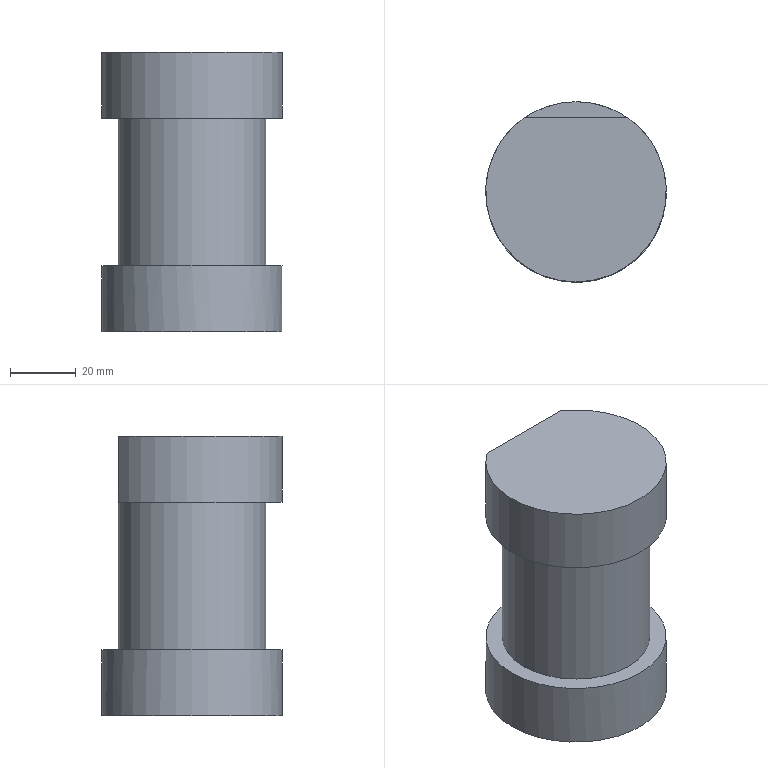Part | NX | features solid 2 | 1 solid | 11 faces | box 55 x 55 x 85 mm | volume 132305 mm3 | plane 6 | cylinder 4 | cone 1 | commonest cylinder face diameters 55 x2 24 x1 45 x1
STEP:
#1=CARTESIAN_POINT('',(690.,-642.5,100.));
#2=VERTEX_POINT('',#1);
#3=CARTESIAN_POINT('',(690.,-665.,100.));
#4=DIRECTION('',(0.,0.,1.));
#5=DIRECTION('',(1.,0.,0.));
#6=AXIS2_PLACEMENT_3D('',#3,#4,#5);
#7=CIRCLE('',#6,22.5);
#8=EDGE_CURVE('',#2,#2,#7,.T.);
#9=ORIENTED_EDGE('',*,*,#8,.F.);
#10=EDGE_LOOP('',(#9));
#11=FACE_BOUND('',#10,.T.);
#12=CARTESIAN_POINT('',(667.5,-665.,55.));
#13=VERTEX_POINT('',#12);
#14=CARTESIAN_POINT('',(690.,-665.,55.));
#15=DIRECTION('',(0.,0.,-1.));
#16=DIRECTION('',(-1.,0.,0.));
#17=AXIS2_PLACEMENT_3D('',#14,#15,#16);
#18=CIRCLE('',#17,22.5);
#19=EDGE_CURVE('',#13,#13,#18,.F.);
#20=ORIENTED_EDGE('',*,*,#19,.T.);
#21=EDGE_LOOP('',(#20));
#22=FACE_BOUND('',#21,.T.);
#23=CARTESIAN_POINT('',(690.,-665.,55.));
#24=DIRECTION('',(0.,0.,1.));
#25=DIRECTION('',(-1.,0.,0.));
#26=AXIS2_PLACEMENT_3D('',#23,#24,#25);
#27=CYLINDRICAL_SURFACE('',#26,22.5);
#28=ADVANCED_FACE('',(#11,#22),#27,.T.);
#29=ORIENTED_EDGE('',*,*,#19,.F.);
#30=EDGE_LOOP('',(#29));
#31=FACE_BOUND('',#30,.T.);
#32=CARTESIAN_POINT('',(717.5,-665.,55.));
#33=VERTEX_POINT('',#32);
#34=CARTESIAN_POINT('',(690.,-665.,55.));
#35=DIRECTION('',(0.,0.,1.));
#36=DIRECTION('',(1.,0.,0.));
#37=AXIS2_PLACEMENT_3D('',#34,#35,#36);
#38=CIRCLE('',#37,27.5);
#39=EDGE_CURVE('',#33,#33,#38,.T.);
#40=ORIENTED_EDGE('',*,*,#39,.T.);
#41=EDGE_LOOP('',(#40));
#42=FACE_BOUND('',#41,.T.);
#43=CARTESIAN_POINT('',(690.,-665.,55.));
#44=DIRECTION('',(0.,0.,1.));
#45=DIRECTION('',(-1.,0.,0.));
#46=AXIS2_PLACEMENT_3D('',#43,#44,#45);
#47=PLANE('',#46);
#48=ADVANCED_FACE('',(#31,#42),#47,.T.);
#49=CARTESIAN_POINT('',(672.,-665.,35.));
#50=VERTEX_POINT('',#49);
#51=CARTESIAN_POINT('',(690.,-665.,35.));
#52=DIRECTION('',(0.,0.,-1.));
#53=DIRECTION('',(-1.,0.,0.));
#54=AXIS2_PLACEMENT_3D('',#51,#52,#53);
#55=CIRCLE('',#54,18.);
#56=EDGE_CURVE('',#50,#50,#55,.T.);
#57=ORIENTED_EDGE('',*,*,#56,.F.);
#58=EDGE_LOOP('',(#57));
#59=FACE_BOUND('',#58,.T.);
#60=CARTESIAN_POINT('',(662.5,-665.,35.));
#61=VERTEX_POINT('',#60);
#62=CARTESIAN_POINT('',(690.,-665.,35.));
#63=DIRECTION('',(0.,0.,-1.));
#64=DIRECTION('',(-1.,0.,0.));
#65=AXIS2_PLACEMENT_3D('',#62,#63,#64);
#66=CIRCLE('',#65,27.5);
#67=EDGE_CURVE('',#61,#61,#66,.T.);
#68=ORIENTED_EDGE('',*,*,#67,.T.);
#69=EDGE_LOOP('',(#68));
#70=FACE_BOUND('',#69,.T.);
#71=CARTESIAN_POINT('',(690.,-665.,35.));
#72=DIRECTION('',(0.,0.,-1.));
#73=DIRECTION('',(1.,0.,0.));
#74=AXIS2_PLACEMENT_3D('',#71,#72,#73);
#75=PLANE('',#74);
#76=ADVANCED_FACE('',(#59,#70),#75,.T.);
#77=ORIENTED_EDGE('',*,*,#39,.F.);
#78=EDGE_LOOP('',(#77));
#79=FACE_BOUND('',#78,.T.);
#80=ORIENTED_EDGE('',*,*,#67,.F.);
#81=EDGE_LOOP('',(#80));
#82=FACE_BOUND('',#81,.T.);
#83=CARTESIAN_POINT('',(690.,-665.,35.));
#84=DIRECTION('',(0.,0.,1.));
#85=DIRECTION('',(-1.,0.,0.));
#86=AXIS2_PLACEMENT_3D('',#83,#84,#85);
#87=CYLINDRICAL_SURFACE('',#86,27.5);
#88=ADVANCED_FACE('',(#79,#82),#87,.T.);
#89=CARTESIAN_POINT('',(705.811,-642.5,100.));
#90=VERTEX_POINT('',#89);
#91=CARTESIAN_POINT('',(690.,-642.5,100.));
#92=DIRECTION('',(1.,0.,0.));
#93=VECTOR('',#92,1000.);
#94=LINE('',#91,#93);
#95=EDGE_CURVE('',#2,#90,#94,.T.);
#96=ORIENTED_EDGE('',*,*,#95,.T.);
#97=CARTESIAN_POINT('',(674.189,-642.5,100.));
#98=VERTEX_POINT('',#97);
#99=CARTESIAN_POINT('',(690.,-665.,100.));
#100=DIRECTION('',(0.,0.,-1.));
#101=DIRECTION('',(-1.,0.,0.));
#102=AXIS2_PLACEMENT_3D('',#99,#100,#101);
#103=CIRCLE('',#102,27.5);
#104=EDGE_CURVE('',#90,#98,#103,.T.);
#105=ORIENTED_EDGE('',*,*,#104,.T.);
#106=CARTESIAN_POINT('',(690.,-642.5,100.));
#107=DIRECTION('',(1.,0.,0.));
#108=VECTOR('',#107,1000.);
#109=LINE('',#106,#108);
#110=EDGE_CURVE('',#98,#2,#109,.T.);
#111=ORIENTED_EDGE('',*,*,#110,.T.);
#112=ORIENTED_EDGE('',*,*,#8,.T.);
#113=EDGE_LOOP('',(#96,#105,#111,#112));
#114=FACE_BOUND('',#113,.T.);
#115=CARTESIAN_POINT('',(690.,-665.,100.));
#116=DIRECTION('',(0.,0.,-1.));
#117=DIRECTION('',(1.,0.,0.));
#118=AXIS2_PLACEMENT_3D('',#115,#116,#117);
#119=PLANE('',#118);
#120=ADVANCED_FACE('',(#114),#119,.T.);
#121=CARTESIAN_POINT('',(705.811,-642.5,120.));
#122=VERTEX_POINT('',#121);
#123=CARTESIAN_POINT('',(674.189,-642.5,120.));
#124=VERTEX_POINT('',#123);
#125=CARTESIAN_POINT('',(690.,-642.5,120.));
#126=DIRECTION('',(-1.,0.,0.));
#127=VECTOR('',#126,1000.);
#128=LINE('',#125,#127);
#129=EDGE_CURVE('',#122,#124,#128,.T.);
#130=ORIENTED_EDGE('',*,*,#129,.T.);
#131=CARTESIAN_POINT('',(690.,-665.,120.));
#132=DIRECTION('',(0.,0.,1.));
#133=DIRECTION('',(1.,0.,0.));
#134=AXIS2_PLACEMENT_3D('',#131,#132,#133);
#135=CIRCLE('',#134,27.5);
#136=EDGE_CURVE('',#124,#122,#135,.T.);
#137=ORIENTED_EDGE('',*,*,#136,.T.);
#138=EDGE_LOOP('',(#130,#137));
#139=FACE_BOUND('',#138,.T.);
#140=CARTESIAN_POINT('',(690.,-665.,120.));
#141=DIRECTION('',(0.,0.,1.));
#142=DIRECTION('',(-1.,0.,0.));
#143=AXIS2_PLACEMENT_3D('',#140,#141,#142);
#144=PLANE('',#143);
#145=ADVANCED_FACE('',(#139),#144,.T.);
#146=CARTESIAN_POINT('',(674.189,-642.5,100.));
#147=DIRECTION('',(0.,0.,1.));
#148=VECTOR('',#147,1000.);
#149=LINE('',#146,#148);
#150=EDGE_CURVE('',#124,#98,#149,.F.);
#151=ORIENTED_EDGE('',*,*,#150,.T.);
#152=ORIENTED_EDGE('',*,*,#104,.F.);
#153=CARTESIAN_POINT('',(705.811,-642.5,100.));
#154=DIRECTION('',(0.,0.,1.));
#155=VECTOR('',#154,1000.);
#156=LINE('',#153,#155);
#157=EDGE_CURVE('',#90,#122,#156,.T.);
#158=ORIENTED_EDGE('',*,*,#157,.T.);
#159=ORIENTED_EDGE('',*,*,#136,.F.);
#160=EDGE_LOOP('',(#151,#152,#158,#159));
#161=FACE_BOUND('',#160,.T.);
#162=CARTESIAN_POINT('',(690.,-665.,100.));
#163=DIRECTION('',(0.,0.,1.));
#164=DIRECTION('',(-1.,0.,0.));
#165=AXIS2_PLACEMENT_3D('',#162,#163,#164);
#166=CYLINDRICAL_SURFACE('',#165,27.5);
#167=ADVANCED_FACE('',(#161),#166,.T.);
#168=ORIENTED_EDGE('',*,*,#150,.F.);
#169=ORIENTED_EDGE('',*,*,#129,.F.);
#170=ORIENTED_EDGE('',*,*,#157,.F.);
#171=ORIENTED_EDGE('',*,*,#95,.F.);
#172=ORIENTED_EDGE('',*,*,#110,.F.);
#173=EDGE_LOOP('',(#168,#169,#170,#171,#172));
#174=FACE_BOUND('',#173,.T.);
#175=CARTESIAN_POINT('',(740.,-642.5,90.));
#176=DIRECTION('',(0.,-1.,0.));
#177=DIRECTION('',(1.,0.,0.));
#178=AXIS2_PLACEMENT_3D('',#175,#176,#177);
#179=PLANE('',#178);
#180=ADVANCED_FACE('',(#174),#179,.F.);
#181=ORIENTED_EDGE('',*,*,#56,.T.);
#182=EDGE_LOOP('',(#181));
#183=FACE_BOUND('',#182,.T.);
#184=CARTESIAN_POINT('',(702.,-665.,45.392));
#185=VERTEX_POINT('',#184);
#186=CARTESIAN_POINT('',(690.,-665.,45.392));
#187=DIRECTION('',(0.,0.,1.));
#188=DIRECTION('',(1.,0.,0.));
#189=AXIS2_PLACEMENT_3D('',#186,#187,#188);
#190=CIRCLE('',#189,12.);
#191=EDGE_CURVE('',#185,#185,#190,.T.);
#192=ORIENTED_EDGE('',*,*,#191,.T.);
#193=EDGE_LOOP('',(#192));
#194=FACE_BOUND('',#193,.T.);
#195=CARTESIAN_POINT('',(690.,-665.,66.177));
#196=DIRECTION('',(0.,0.,-1.));
#197=DIRECTION('',(1.,0.,0.));
#198=AXIS2_PLACEMENT_3D('',#195,#196,#197);
#199=CONICAL_SURFACE('',#198,0.,0.5236);
#200=ADVANCED_FACE('',(#183,#194),#199,.F.);
#201=CARTESIAN_POINT('',(702.,-665.,100.));
#202=VERTEX_POINT('',#201);
#203=CARTESIAN_POINT('',(690.,-665.,100.));
#204=DIRECTION('',(0.,0.,1.));
#205=DIRECTION('',(1.,0.,0.));
#206=AXIS2_PLACEMENT_3D('',#203,#204,#205);
#207=CIRCLE('',#206,12.);
#208=EDGE_CURVE('',#202,#202,#207,.T.);
#209=ORIENTED_EDGE('',*,*,#208,.F.);
#210=EDGE_LOOP('',(#209));
#211=FACE_BOUND('',#210,.T.);
#212=CARTESIAN_POINT('',(690.,-665.,100.));
#213=DIRECTION('',(0.,0.,1.));
#214=DIRECTION('',(-1.,0.,0.));
#215=AXIS2_PLACEMENT_3D('',#212,#213,#214);
#216=PLANE('',#215);
#217=ADVANCED_FACE('',(#211),#216,.F.);
#218=ORIENTED_EDGE('',*,*,#191,.F.);
#219=EDGE_LOOP('',(#218));
#220=FACE_BOUND('',#219,.T.);
#221=ORIENTED_EDGE('',*,*,#208,.T.);
#222=EDGE_LOOP('',(#221));
#223=FACE_BOUND('',#222,.T.);
#224=CARTESIAN_POINT('',(690.,-665.,35.));
#225=DIRECTION('',(0.,0.,1.));
#226=DIRECTION('',(-1.,0.,0.));
#227=AXIS2_PLACEMENT_3D('',#224,#225,#226);
#228=CYLINDRICAL_SURFACE('',#227,12.);
#229=ADVANCED_FACE('',(#220,#223),#228,.F.);
#230=CLOSED_SHELL('',(#28,#48,#76,#88,#120,#145,#167,#180,#200,#217,#229));
#231=MANIFOLD_SOLID_BREP('',#230);
#232=(LENGTH_UNIT()NAMED_UNIT(*)SI_UNIT(.MILLI.,.METRE.));
#233=UNCERTAINTY_MEASURE_WITH_UNIT(LENGTH_MEASURE(0.00001),#232,'','');
#234=(NAMED_UNIT(*)PLANE_ANGLE_UNIT()SI_UNIT($,.RADIAN.));
#235=(NAMED_UNIT(*)SI_UNIT($,.STERADIAN.)SOLID_ANGLE_UNIT());
#236=(GEOMETRIC_REPRESENTATION_CONTEXT(3)GLOBAL_UNCERTAINTY_ASSIGNED_CONTEXT((#233))GLOBAL_UNIT_ASSIGNED_CONTEXT((#232,#234,#235))REPRESENTATION_CONTEXT('',''));
#237=ADVANCED_BREP_SHAPE_REPRESENTATION('',(#231),#236);